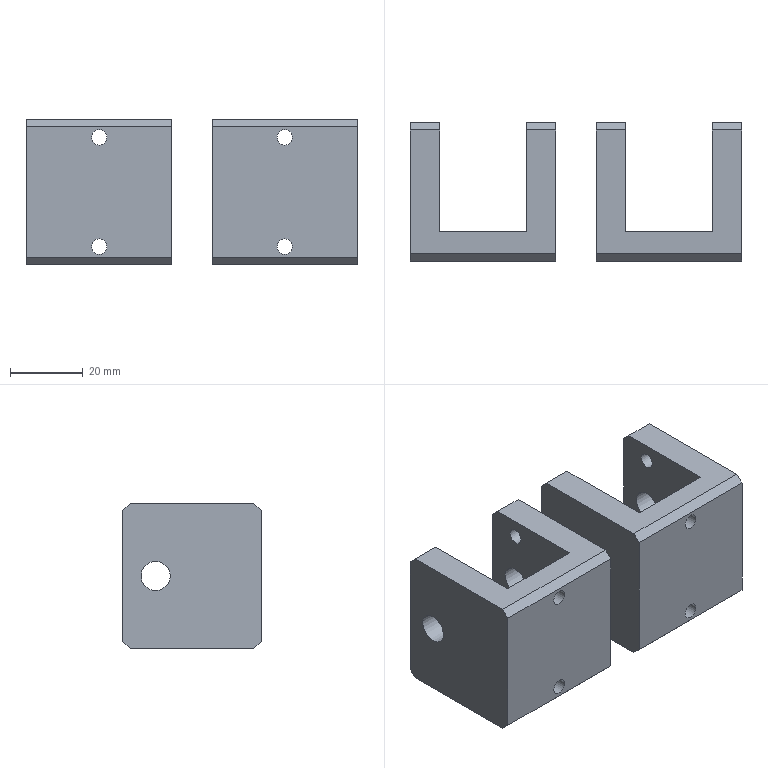NC program | NX | posted by the shop | part box 91 x 38 x 40 mm
Lines 1 to 3675 of 4199, first 2229 of 3673 lines:
%
O0001
(Machine time: 136.35 MIN)
(===Total Tool:6===)
(T1=D80R0.8 face mill D=80.  R=0.8  D-  H01 Z=-0.   )
(T9=D10     D=10.  R=0.   D-  H09 Z=-38.1 )
(T2=D6 chamfer mill   D=6.   R=0.   D-  H02 Z=-31.5 )
(T14=Drill 4.2  D=4.2  DR_a=118 D-  H14 Z=-45.26)
(T10=D10-J  D=10.  R=0.   D-  H10 Z=-38.  )
(T22=M5X0.8 D=4.2  DR_a=180 D-  H22 Z=-41.5 )
G80 G90 G17 G49 G40
G91 G28 Z0
M01
N1 T01 M06
(D80R0.8 face mill  D=80. R=0.8 H=01 ce=0.00 di=0.00)
G00 G90 G54 X90.5 Y0.0 M03 S4000
G43 H01 Z50.
M08
Z2.
G01 Z0.0 F1000.
X85.5
X-85.5
X-90.5
Z2.
G00 Z50.
G91 G28 Z0.0
M05
M09
G91 G28 Z0.0
M01
N2 T09 M06
(D10  D=10. R=0. H=09 ce=0.10 di=0.00)
G00 G90 G54 X50.6 Y0.0 M03 S8000
G43 H09 Z50.
M08
Z.5
G01 Y-20. Z.418 F5000.
G02 X45.5 Y-25.1 Z.385 I-5.1 J0.0
G01 X5.5 Z.221
G02 X.4 Y-20. Z.188 I0.0 J5.1
G01 Y20. Z.024
G02 X5.5 Y25.1 Z-.009 I5.1 J0.0
G01 X45.5 Z-.173
G02 X50.6 Y20. Z-.206 I0.0 J-5.1
G01 Y-20. Z-.37
G02 X45.5 Y-25.1 Z-.403 I-5.1 J0.0
G01 X5.5 Z-.567
G02 X.4 Y-20. Z-.6 I0.0 J5.1
G01 Y20. Z-.764
G02 X5.5 Y25.1 Z-.797 I5.1 J0.0
G01 X45.5 Z-.961
G02 X50.6 Y20. Z-.993 I0.0 J-5.1
G01 Y-20. Z-1.158
G02 X45.5 Y-25.1 Z-1.19 I-5.1 J0.0
G01 X5.5 Z-1.354
G02 X.4 Y-20. Z-1.387 I0.0 J5.1
G01 Y20. Z-1.551
G02 X5.5 Y25.1 Z-1.584 I5.1 J0.0
G01 X45.5 Z-1.748
G02 X50.6 Y20. Z-1.781 I0.0 J-5.1
G01 Y-20. Z-1.945
G02 X45.5 Y-25.1 Z-1.978 I-5.1 J0.0
G01 X5.5 Z-2.142
G02 X.4 Y-20. Z-2.175 I0.0 J5.1
G01 Y20. Z-2.339
G02 X5.5 Y25.1 Z-2.372 I5.1 J0.0
G01 X45.5 Z-2.536
G02 X50.6 Y20. Z-2.569 I0.0 J-5.1
G01 Y-20. Z-2.733
G02 X45.5 Y-25.1 Z-2.766 I-5.1 J0.0
G01 X5.5 Z-2.93
G02 X.4 Y-20. Z-2.963 I0.0 J5.1
G01 Y20. Z-3.127
G02 X5.5 Y25.1 Z-3.16 I5.1 J0.0
G01 X45.5 Z-3.324
G02 X50.6 Y20. Z-3.357 I0.0 J-5.1
G01 Y-20. Z-3.521
G02 X45.5 Y-25.1 Z-3.554 I-5.1 J0.0
G01 X5.5 Z-3.718
G02 X.4 Y-20. Z-3.751 I0.0 J5.1
G01 Y20. Z-3.915
G02 X5.5 Y25.1 Z-3.948 I5.1 J0.0
G01 X45.5 Z-4.112
G02 X50.6 Y20. Z-4.144 I0.0 J-5.1
G01 Y-20. Z-4.309
G02 X45.5 Y-25.1 Z-4.341 I-5.1 J0.0
G01 X5.5 Z-4.506
G02 X.4 Y-20. Z-4.538 I0.0 J5.1
G01 Y20. Z-4.702
G02 X5.5 Y25.1 Z-4.735 I5.1 J0.0
G01 X45.5 Z-4.899
G02 X50.6 Y20. Z-4.932 I0.0 J-5.1
G01 Y-20. Z-5.096
G02 X45.5 Y-25.1 Z-5.129 I-5.1 J0.0
G01 X5.5 Z-5.293
G02 X.4 Y-20. Z-5.326 I0.0 J5.1
G01 Y20. Z-5.49
G02 X5.5 Y25.1 Z-5.523 I5.1 J0.0
G01 X45.5 Z-5.687
G02 X50.6 Y20. Z-5.72 I0.0 J-5.1
G01 Y-20. Z-5.884
G02 X45.5 Y-25.1 Z-5.917 I-5.1 J0.0
G01 X5.5 Z-6.081
G02 X.4 Y-20. Z-6.114 I0.0 J5.1
G01 Y20. Z-6.278
G02 X5.5 Y25.1 Z-6.311 I5.1 J0.0
G01 X45.5 Z-6.475
G02 X50.6 Y20. Z-6.508 I0.0 J-5.1
G01 Y-20. Z-6.672
G02 X45.5 Y-25.1 Z-6.705 I-5.1 J0.0
G01 X5.5 Z-6.869
G02 X.4 Y-20. Z-6.902 I0.0 J5.1
G01 Y20. Z-7.066
G02 X5.5 Y25.1 Z-7.099 I5.1 J0.0
G01 X45.5 Z-7.263
G02 X50.6 Y20. Z-7.296 I0.0 J-5.1
G01 Y-20. Z-7.46
G02 X45.5 Y-25.1 Z-7.492 I-5.1 J0.0
G01 X5.5 Z-7.657
G02 X.4 Y-20. Z-7.689 I0.0 J5.1
G01 Y20. Z-7.853
G02 X5.5 Y25.1 Z-7.886 I5.1 J0.0
G01 X45.5 Z-8.05
G02 X50.6 Y20. Z-8.083 I0.0 J-5.1
G01 Y-20. Z-8.247
G02 X45.5 Y-25.1 Z-8.28 I-5.1 J0.0
G01 X5.5 Z-8.444
G02 X.4 Y-20. Z-8.477 I0.0 J5.1
G01 Y20. Z-8.641
G02 X5.5 Y25.1 Z-8.674 I5.1 J0.0
G01 X45.5 Z-8.838
G02 X50.6 Y20. Z-8.871 I0.0 J-5.1
G01 Y-20. Z-9.035
G02 X45.5 Y-25.1 Z-9.068 I-5.1 J0.0
G01 X5.5 Z-9.232
G02 X.4 Y-20. Z-9.265 I0.0 J5.1
G01 Y20. Z-9.429
G02 X5.5 Y25.1 Z-9.462 I5.1 J0.0
G01 X45.5 Z-9.626
G02 X50.6 Y20. Z-9.659 I0.0 J-5.1
G01 Y-20. Z-9.823
G02 X45.5 Y-25.1 Z-9.856 I-5.1 J0.0
G01 X5.5 Z-10.02
G02 X.4 Y-20. Z-10.053 I0.0 J5.1
G01 Y20. Z-10.217
G02 X5.5 Y25.1 Z-10.25 I5.1 J0.0
G01 X45.5 Z-10.414
G02 X50.6 Y20. Z-10.447 I0.0 J-5.1
G01 Y-20. Z-10.611
G02 X45.5 Y-25.1 Z-10.643 I-5.1 J0.0
G01 X5.5 Z-10.808
G02 X.4 Y-20. Z-10.84 I0.0 J5.1
G01 Y20. Z-11.004
G02 X5.5 Y25.1 Z-11.037 I5.1 J0.0
G01 X45.5 Z-11.201
G02 X50.6 Y20. Z-11.234 I0.0 J-5.1
G01 Y-20. Z-11.398
G02 X45.5 Y-25.1 Z-11.431 I-5.1 J0.0
G01 X5.5 Z-11.595
G02 X.4 Y-20. Z-11.628 I0.0 J5.1
G01 Y20. Z-11.792
G02 X5.5 Y25.1 Z-11.825 I5.1 J0.0
G01 X45.5 Z-11.989
G02 X50.6 Y20. Z-12.022 I0.0 J-5.1
G01 Y-20. Z-12.186
G02 X45.5 Y-25.1 Z-12.219 I-5.1 J0.0
G01 X5.5 Z-12.383
G02 X.4 Y-20. Z-12.416 I0.0 J5.1
G01 Y20. Z-12.58
G02 X5.5 Y25.1 Z-12.613 I5.1 J0.0
G01 X45.5 Z-12.777
G02 X50.6 Y20. Z-12.81 I0.0 J-5.1
G01 Y-20. Z-12.974
G02 X45.5 Y-25.1 Z-13.007 I-5.1 J0.0
G01 X5.5 Z-13.171
G02 X.4 Y-20. Z-13.204 I0.0 J5.1
G01 Y20. Z-13.368
G02 X5.5 Y25.1 Z-13.401 I5.1 J0.0
G01 X45.5 Z-13.565
G02 X50.6 Y20. Z-13.598 I0.0 J-5.1
G01 Y-20. Z-13.762
G02 X45.5 Y-25.1 Z-13.794 I-5.1 J0.0
G01 X5.5 Z-13.959
G02 X.4 Y-20. Z-13.991 I0.0 J5.1
G01 Y20. Z-14.156
G02 X5.5 Y25.1 Z-14.188 I5.1 J0.0
G01 X45.5 Z-14.352
G02 X50.6 Y20. Z-14.385 I0.0 J-5.1
G01 Y-20. Z-14.549
G02 X45.5 Y-25.1 Z-14.582 I-5.1 J0.0
G01 X5.5 Z-14.746
G02 X.4 Y-20. Z-14.779 I0.0 J5.1
G01 Y20. Z-14.943
G02 X5.5 Y25.1 Z-14.976 I5.1 J0.0
G01 X45.5 Z-15.14
G02 X50.6 Y20. Z-15.173 I0.0 J-5.1
G01 Y-20. Z-15.337
G02 X45.5 Y-25.1 Z-15.37 I-5.1 J0.0
G01 X5.5 Z-15.534
G02 X.4 Y-20. Z-15.567 I0.0 J5.1
G01 Y20. Z-15.731
G02 X5.5 Y25.1 Z-15.764 I5.1 J0.0
G01 X45.5 Z-15.928
G02 X50.6 Y20. Z-15.961 I0.0 J-5.1
G01 Y-20. Z-16.125
G02 X45.5 Y-25.1 Z-16.158 I-5.1 J0.0
G01 X5.5 Z-16.322
G02 X.4 Y-20. Z-16.355 I0.0 J5.1
G01 Y20. Z-16.519
G02 X5.5 Y25.1 Z-16.552 I5.1 J0.0
G01 X45.5 Z-16.716
G02 X50.6 Y20. Z-16.749 I0.0 J-5.1
G01 Y-20. Z-16.913
G02 X45.5 Y-25.1 Z-16.946 I-5.1 J0.0
G01 X5.5 Z-17.11
G02 X.4 Y-20. Z-17.142 I0.0 J5.1
G01 Y20. Z-17.307
G02 X5.5 Y25.1 Z-17.339 I5.1 J0.0
G01 X45.5 Z-17.503
G02 X50.6 Y20. Z-17.536 I0.0 J-5.1
G01 Y-20. Z-17.7
G02 X45.5 Y-25.1 Z-17.733 I-5.1 J0.0
G01 X5.5 Z-17.897
G02 X.4 Y-20. Z-17.93 I0.0 J5.1
G01 Y20. Z-18.094
G02 X5.5 Y25.1 Z-18.127 I5.1 J0.0
G01 X45.5 Z-18.291
G02 X50.6 Y20. Z-18.324 I0.0 J-5.1
G01 Y-20. Z-18.488
G02 X45.5 Y-25.1 Z-18.521 I-5.1 J0.0
G01 X5.5 Z-18.685
G02 X.4 Y-20. Z-18.718 I0.0 J5.1
G01 Y20. Z-18.882
G02 X5.5 Y25.1 Z-18.915 I5.1 J0.0
G01 X45.5 Z-19.079
G02 X50.6 Y20. Z-19.112 I0.0 J-5.1
G01 Y-20. Z-19.276
G02 X45.5 Y-25.1 Z-19.309 I-5.1 J0.0
G01 X5.5 Z-19.473
G02 X.4 Y-20. Z-19.506 I0.0 J5.1
G01 Y20. Z-19.67
G02 X5.5 Y25.1 Z-19.703 I5.1 J0.0
G01 X45.5 Z-19.867
G02 X50.6 Y20. Z-19.9 I0.0 J-5.1
G01 Y-20. Z-20.064
G02 X45.5 Y-25.1 Z-20.097 I-5.1 J0.0
G01 X5.5 Z-20.261
G02 X.4 Y-20. Z-20.293 I0.0 J5.1
G01 Y20. Z-20.458
G02 X5.5 Y25.1 Z-20.49 I5.1 J0.0
G01 X45.5 Z-20.654
G02 X50.6 Y20. Z-20.687 I0.0 J-5.1
G01 Y-20. Z-20.851
G02 X45.5 Y-25.1 Z-20.884 I-5.1 J0.0
G01 X5.5 Z-21.048
G02 X.4 Y-20. Z-21.081 I0.0 J5.1
G01 Y20. Z-21.245
G02 X5.5 Y25.1 Z-21.278 I5.1 J0.0
G01 X45.5 Z-21.442
G02 X50.6 Y20. Z-21.475 I0.0 J-5.1
G01 Y-20. Z-21.639
G02 X45.5 Y-25.1 Z-21.672 I-5.1 J0.0
G01 X5.5 Z-21.836
G02 X.4 Y-20. Z-21.869 I0.0 J5.1
G01 Y20. Z-22.033
G02 X5.5 Y25.1 Z-22.066 I5.1 J0.0
G01 X45.5 Z-22.23
G02 X50.6 Y20. Z-22.263 I0.0 J-5.1
G01 Y-20. Z-22.427
G02 X45.5 Y-25.1 Z-22.46 I-5.1 J0.0
G01 X5.5 Z-22.624
G02 X.4 Y-20. Z-22.657 I0.0 J5.1
G01 Y20. Z-22.821
G02 X5.5 Y25.1 Z-22.854 I5.1 J0.0
G01 X45.5 Z-23.018
G02 X50.6 Y20. Z-23.051 I0.0 J-5.1
G01 Y-20. Z-23.215
G02 X45.5 Y-25.1 Z-23.248 I-5.1 J0.0
G01 X5.5 Z-23.412
G02 X.4 Y-20. Z-23.444 I0.0 J5.1
G01 Y20. Z-23.609
G02 X5.5 Y25.1 Z-23.641 I5.1 J0.0
G01 X45.5 Z-23.806
G02 X50.6 Y20. Z-23.838 I0.0 J-5.1
G01 Y-20. Z-24.002
G02 X45.5 Y-25.1 Z-24.035 I-5.1 J0.0
G01 X5.5 Z-24.199
G02 X.4 Y-20. Z-24.232 I0.0 J5.1
G01 Y20. Z-24.396
G02 X5.5 Y25.1 Z-24.429 I5.1 J0.0
G01 X45.5 Z-24.593
G02 X50.6 Y20. Z-24.626 I0.0 J-5.1
G01 Y-20. Z-24.79
G02 X45.5 Y-25.1 Z-24.823 I-5.1 J0.0
G01 X5.5 Z-24.987
G02 X.4 Y-20. Z-25.02 I0.0 J5.1
G01 Y20. Z-25.184
G02 X5.5 Y25.1 Z-25.217 I5.1 J0.0
G01 X45.5 Z-25.381
G02 X50.6 Y20. Z-25.414 I0.0 J-5.1
G01 Y-20. Z-25.578
G02 X45.5 Y-25.1 Z-25.611 I-5.1 J0.0
G01 X5.5 Z-25.775
G02 X.4 Y-20. Z-25.808 I0.0 J5.1
G01 Y20. Z-25.972
G02 X5.5 Y25.1 Z-26.005 I5.1 J0.0
G01 X45.5 Z-26.169
G02 X50.6 Y20. Z-26.202 I0.0 J-5.1
G01 Y-20. Z-26.366
G02 X45.5 Y-25.1 Z-26.399 I-5.1 J0.0
G01 X5.5 Z-26.563
G02 X.4 Y-20. Z-26.596 I0.0 J5.1
G01 Y20. Z-26.76
G02 X5.5 Y25.1 Z-26.792 I5.1 J0.0
G01 X45.5 Z-26.957
G02 X50.6 Y20. Z-26.989 I0.0 J-5.1
G01 Y-20. Z-27.153
G02 X45.5 Y-25.1 Z-27.186 I-5.1 J0.0
G01 X5.5 Z-27.35
G02 X.4 Y-20. Z-27.383 I0.0 J5.1
G01 Y20. Z-27.547
G02 X5.5 Y25.1 Z-27.58 I5.1 J0.0
G01 X45.5 Z-27.744
G02 X50.6 Y20. Z-27.777 I0.0 J-5.1
G01 Y-20. Z-27.941
G02 X45.5 Y-25.1 Z-27.974 I-5.1 J0.0
G01 X5.5 Z-28.138
G02 X.4 Y-20. Z-28.171 I0.0 J5.1
G01 Y20. Z-28.335
G02 X5.5 Y25.1 Z-28.368 I5.1 J0.0
G01 X45.5 Z-28.532
G02 X50.6 Y20. Z-28.565 I0.0 J-5.1
G01 Y-20. Z-28.729
G02 X45.5 Y-25.1 Z-28.762 I-5.1 J0.0
G01 X5.5 Z-28.926
G02 X.4 Y-20. Z-28.959 I0.0 J5.1
G01 Y20. Z-29.123
G02 X5.5 Y25.1 Z-29.156 I5.1 J0.0
G01 X45.5 Z-29.32
G02 X50.6 Y20. Z-29.353 I0.0 J-5.1
G01 Y-20. Z-29.517
G02 X45.5 Y-25.1 Z-29.55 I-5.1 J0.0
G01 X5.5 Z-29.714
G02 X.4 Y-20. Z-29.747 I0.0 J5.1
G01 Y20. Z-29.911
G02 X5.5 Y25.1 Z-29.943 I5.1 J0.0
G01 X45.5 Z-30.108
G02 X50.6 Y20. Z-30.14 I0.0 J-5.1
G01 Y-20. Z-30.304
G02 X45.5 Y-25.1 Z-30.337 I-5.1 J0.0
G01 X5.5 Z-30.501
G02 X.4 Y-20. Z-30.534 I0.0 J5.1
G01 Y20. Z-30.698
G02 X5.5 Y25.1 Z-30.731 I5.1 J0.0
G01 X45.5 Z-30.895
G02 X50.6 Y20. Z-30.928 I0.0 J-5.1
G01 Y-20. Z-31.092
G02 X45.5 Y-25.1 Z-31.125 I-5.1 J0.0
G01 X5.5 Z-31.289
G02 X.4 Y-20. Z-31.322 I0.0 J5.1
G01 Y20. Z-31.486
G02 X5.5 Y25.1 Z-31.519 I5.1 J0.0
G01 X45.5 Z-31.683
G02 X50.6 Y20. Z-31.716 I0.0 J-5.1
G01 Y-20. Z-31.88
G02 X45.5 Y-25.1 Z-31.913 I-5.1 J0.0
G01 X5.5 Z-32.077
G02 X.4 Y-20. Z-32.11 I0.0 J5.1
G01 Y20. Z-32.274
G02 X5.5 Y25.1 Z-32.307 I5.1 J0.0
G01 X45.5 Z-32.471
G02 X50.6 Y20. Z-32.504 I0.0 J-5.1
G01 Y-20. Z-32.668
G02 X45.5 Y-25.1 Z-32.701 I-5.1 J0.0
G01 X5.5 Z-32.865
G02 X.4 Y-20. Z-32.898 I0.0 J5.1
G01 Y20. Z-33.062
G02 X5.5 Y25.1 Z-33.094 I5.1 J0.0
G01 X45.5 Z-33.259
G02 X50.6 Y20. Z-33.291 I0.0 J-5.1
G01 Y-20. Z-33.456
G02 X45.5 Y-25.1 Z-33.488 I-5.1 J0.0
G01 X5.5 Z-33.652
G02 X.4 Y-20. Z-33.685 I0.0 J5.1
G01 Y20. Z-33.849
G02 X5.5 Y25.1 Z-33.882 I5.1 J0.0
G01 X45.5 Z-34.046
G02 X50.6 Y20. Z-34.079 I0.0 J-5.1
G01 Y-20. Z-34.243
G02 X45.5 Y-25.1 Z-34.276 I-5.1 J0.0
G01 X5.5 Z-34.44
G02 X.4 Y-20. Z-34.473 I0.0 J5.1
G01 Y20. Z-34.637
G02 X5.5 Y25.1 Z-34.67 I5.1 J0.0
G01 X45.5 Z-34.834
G02 X50.6 Y20. Z-34.867 I0.0 J-5.1
G01 Y-20. Z-35.031
G02 X45.5 Y-25.1 Z-35.064 I-5.1 J0.0
G01 X5.5 Z-35.228
G02 X.4 Y-20. Z-35.261 I0.0 J5.1
G01 Y20. Z-35.425
G02 X5.5 Y25.1 Z-35.458 I5.1 J0.0
G01 X45.5 Z-35.622
G02 X50.6 Y20. Z-35.655 I0.0 J-5.1
G01 Y-20. Z-35.819
G02 X45.5 Y-25.1 Z-35.852 I-5.1 J0.0
G01 X5.5 Z-36.016
G02 X.4 Y-20. Z-36.049 I0.0 J5.1
G01 Y20. Z-36.213
G02 X5.5 Y25.1 Z-36.246 I5.1 J0.0
G01 X45.5 Z-36.41
G02 X50.6 Y20. Z-36.442 I0.0 J-5.1
G01 Y-20. Z-36.607
G02 X45.5 Y-25.1 Z-36.639 I-5.1 J0.0
G01 X5.5 Z-36.803
G02 X.4 Y-20. Z-36.836 I0.0 J5.1
G01 Y20. Z-37.
G02 X5.5 Y25.1 Z-37.033 I5.1 J0.0
G01 X45.5 Z-37.197
G02 X50.6 Y20. Z-37.23 I0.0 J-5.1
G01 Y-20. Z-37.394
G02 X45.5 Y-25.1 Z-37.427 I-5.1 J0.0
G01 X5.5 Z-37.591
G02 X.4 Y-20. Z-37.624 I0.0 J5.1
G01 Y20. Z-37.788
G02 X5.5 Y25.1 Z-37.821 I5.1 J0.0
G01 X45.5 Z-37.985
G02 X50.6 Y20. Z-38.018 I0.0 J-5.1
G01 Y0.0 Z-38.1
Y-20.
G02 X45.5 Y-25.1 I-5.1 J0.0
G01 X5.5
G02 X.4 Y-20. I0.0 J5.1
G01 Y20.
G02 X5.5 Y25.1 I5.1 J0.0
G01 X45.5
G02 X50.6 Y20. I0.0 J-5.1
G01 Y0.0
Y-.5
Z-37.1
G00 Z50.
X-25.5 Y25.1
Z.5
G01 X-5.5 Z.418
G02 X-.4 Y20. Z.385 I0.0 J-5.1
G01 Y-20. Z.221
G02 X-5.5 Y-25.1 Z.188 I-5.1 J0.0
G01 X-45.5 Z.024
G02 X-50.6 Y-20. Z-.009 I0.0 J5.1
G01 Y20. Z-.173
G02 X-45.5 Y25.1 Z-.206 I5.1 J0.0
G01 X-5.5 Z-.37
G02 X-.4 Y20. Z-.403 I0.0 J-5.1
G01 Y-20. Z-.567
G02 X-5.5 Y-25.1 Z-.6 I-5.1 J0.0
G01 X-45.5 Z-.764
G02 X-50.6 Y-20. Z-.797 I0.0 J5.1
G01 Y20. Z-.961
G02 X-45.5 Y25.1 Z-.993 I5.1 J0.0
G01 X-5.5 Z-1.158
G02 X-.4 Y20. Z-1.19 I0.0 J-5.1
G01 Y-20. Z-1.354
G02 X-5.5 Y-25.1 Z-1.387 I-5.1 J0.0
G01 X-45.5 Z-1.551
G02 X-50.6 Y-20. Z-1.584 I0.0 J5.1
G01 Y20. Z-1.748
G02 X-45.5 Y25.1 Z-1.781 I5.1 J0.0
G01 X-5.5 Z-1.945
G02 X-.4 Y20. Z-1.978 I0.0 J-5.1
G01 Y-20. Z-2.142
G02 X-5.5 Y-25.1 Z-2.175 I-5.1 J0.0
G01 X-45.5 Z-2.339
G02 X-50.6 Y-20. Z-2.372 I0.0 J5.1
G01 Y20. Z-2.536
G02 X-45.5 Y25.1 Z-2.569 I5.1 J0.0
G01 X-5.5 Z-2.733
G02 X-.4 Y20. Z-2.766 I0.0 J-5.1
G01 Y-20. Z-2.93
G02 X-5.5 Y-25.1 Z-2.963 I-5.1 J0.0
G01 X-45.5 Z-3.127
G02 X-50.6 Y-20. Z-3.16 I0.0 J5.1
G01 Y20. Z-3.324
G02 X-45.5 Y25.1 Z-3.357 I5.1 J0.0
G01 X-5.5 Z-3.521
G02 X-.4 Y20. Z-3.554 I0.0 J-5.1
G01 Y-20. Z-3.718
G02 X-5.5 Y-25.1 Z-3.751 I-5.1 J0.0
G01 X-45.5 Z-3.915
G02 X-50.6 Y-20. Z-3.948 I0.0 J5.1
G01 Y20. Z-4.112
G02 X-45.5 Y25.1 Z-4.144 I5.1 J0.0
G01 X-5.5 Z-4.309
G02 X-.4 Y20. Z-4.341 I0.0 J-5.1
G01 Y-20. Z-4.506
G02 X-5.5 Y-25.1 Z-4.538 I-5.1 J0.0
G01 X-45.5 Z-4.702
G02 X-50.6 Y-20. Z-4.735 I0.0 J5.1
G01 Y20. Z-4.899
G02 X-45.5 Y25.1 Z-4.932 I5.1 J0.0
G01 X-5.5 Z-5.096
G02 X-.4 Y20. Z-5.129 I0.0 J-5.1
G01 Y-20. Z-5.293
G02 X-5.5 Y-25.1 Z-5.326 I-5.1 J0.0
G01 X-45.5 Z-5.49
G02 X-50.6 Y-20. Z-5.523 I0.0 J5.1
G01 Y20. Z-5.687
G02 X-45.5 Y25.1 Z-5.72 I5.1 J0.0
G01 X-5.5 Z-5.884
G02 X-.4 Y20. Z-5.917 I0.0 J-5.1
G01 Y-20. Z-6.081
G02 X-5.5 Y-25.1 Z-6.114 I-5.1 J0.0
G01 X-45.5 Z-6.278
G02 X-50.6 Y-20. Z-6.311 I0.0 J5.1
G01 Y20. Z-6.475
G02 X-45.5 Y25.1 Z-6.508 I5.1 J0.0
G01 X-5.5 Z-6.672
G02 X-.4 Y20. Z-6.705 I0.0 J-5.1
G01 Y-20. Z-6.869
G02 X-5.5 Y-25.1 Z-6.902 I-5.1 J0.0
G01 X-45.5 Z-7.066
G02 X-50.6 Y-20. Z-7.099 I0.0 J5.1
G01 Y20. Z-7.263
G02 X-45.5 Y25.1 Z-7.296 I5.1 J0.0
G01 X-5.5 Z-7.46
G02 X-.4 Y20. Z-7.492 I0.0 J-5.1
G01 Y-20. Z-7.657
G02 X-5.5 Y-25.1 Z-7.689 I-5.1 J0.0
G01 X-45.5 Z-7.853
G02 X-50.6 Y-20. Z-7.886 I0.0 J5.1
G01 Y20. Z-8.05
G02 X-45.5 Y25.1 Z-8.083 I5.1 J0.0
G01 X-5.5 Z-8.247
G02 X-.4 Y20. Z-8.28 I0.0 J-5.1
G01 Y-20. Z-8.444
G02 X-5.5 Y-25.1 Z-8.477 I-5.1 J0.0
G01 X-45.5 Z-8.641
G02 X-50.6 Y-20. Z-8.674 I0.0 J5.1
G01 Y20. Z-8.838
G02 X-45.5 Y25.1 Z-8.871 I5.1 J0.0
G01 X-5.5 Z-9.035
G02 X-.4 Y20. Z-9.068 I0.0 J-5.1
G01 Y-20. Z-9.232
G02 X-5.5 Y-25.1 Z-9.265 I-5.1 J0.0
G01 X-45.5 Z-9.429
G02 X-50.6 Y-20. Z-9.462 I0.0 J5.1
G01 Y20. Z-9.626
G02 X-45.5 Y25.1 Z-9.659 I5.1 J0.0
G01 X-5.5 Z-9.823
G02 X-.4 Y20. Z-9.856 I0.0 J-5.1
G01 Y-20. Z-10.02
G02 X-5.5 Y-25.1 Z-10.053 I-5.1 J0.0
G01 X-45.5 Z-10.217
G02 X-50.6 Y-20. Z-10.25 I0.0 J5.1
G01 Y20. Z-10.414
G02 X-45.5 Y25.1 Z-10.447 I5.1 J0.0
G01 X-5.5 Z-10.611
G02 X-.4 Y20. Z-10.643 I0.0 J-5.1
G01 Y-20. Z-10.808
G02 X-5.5 Y-25.1 Z-10.84 I-5.1 J0.0
G01 X-45.5 Z-11.004
G02 X-50.6 Y-20. Z-11.037 I0.0 J5.1
G01 Y20. Z-11.201
G02 X-45.5 Y25.1 Z-11.234 I5.1 J0.0
G01 X-5.5 Z-11.398
G02 X-.4 Y20. Z-11.431 I0.0 J-5.1
G01 Y-20. Z-11.595
G02 X-5.5 Y-25.1 Z-11.628 I-5.1 J0.0
G01 X-45.5 Z-11.792
G02 X-50.6 Y-20. Z-11.825 I0.0 J5.1
G01 Y20. Z-11.989
G02 X-45.5 Y25.1 Z-12.022 I5.1 J0.0
G01 X-5.5 Z-12.186
G02 X-.4 Y20. Z-12.219 I0.0 J-5.1
G01 Y-20. Z-12.383
G02 X-5.5 Y-25.1 Z-12.416 I-5.1 J0.0
G01 X-45.5 Z-12.58
G02 X-50.6 Y-20. Z-12.613 I0.0 J5.1
G01 Y20. Z-12.777
G02 X-45.5 Y25.1 Z-12.81 I5.1 J0.0
G01 X-5.5 Z-12.974
G02 X-.4 Y20. Z-13.007 I0.0 J-5.1
G01 Y-20. Z-13.171
G02 X-5.5 Y-25.1 Z-13.204 I-5.1 J0.0
G01 X-45.5 Z-13.368
G02 X-50.6 Y-20. Z-13.401 I0.0 J5.1
G01 Y20. Z-13.565
G02 X-45.5 Y25.1 Z-13.598 I5.1 J0.0
G01 X-5.5 Z-13.762
G02 X-.4 Y20. Z-13.794 I0.0 J-5.1
G01 Y-20. Z-13.959
G02 X-5.5 Y-25.1 Z-13.991 I-5.1 J0.0
G01 X-45.5 Z-14.156
G02 X-50.6 Y-20. Z-14.188 I0.0 J5.1
G01 Y20. Z-14.352
G02 X-45.5 Y25.1 Z-14.385 I5.1 J0.0
G01 X-5.5 Z-14.549
G02 X-.4 Y20. Z-14.582 I0.0 J-5.1
G01 Y-20. Z-14.746
G02 X-5.5 Y-25.1 Z-14.779 I-5.1 J0.0
G01 X-45.5 Z-14.943
G02 X-50.6 Y-20. Z-14.976 I0.0 J5.1
G01 Y20. Z-15.14
G02 X-45.5 Y25.1 Z-15.173 I5.1 J0.0
G01 X-5.5 Z-15.337
G02 X-.4 Y20. Z-15.37 I0.0 J-5.1
G01 Y-20. Z-15.534
G02 X-5.5 Y-25.1 Z-15.567 I-5.1 J0.0
G01 X-45.5 Z-15.731
G02 X-50.6 Y-20. Z-15.764 I0.0 J5.1
G01 Y20. Z-15.928
G02 X-45.5 Y25.1 Z-15.961 I5.1 J0.0
G01 X-5.5 Z-16.125
G02 X-.4 Y20. Z-16.158 I0.0 J-5.1
G01 Y-20. Z-16.322
G02 X-5.5 Y-25.1 Z-16.355 I-5.1 J0.0
G01 X-45.5 Z-16.519
G02 X-50.6 Y-20. Z-16.552 I0.0 J5.1
G01 Y20. Z-16.716
G02 X-45.5 Y25.1 Z-16.749 I5.1 J0.0
G01 X-5.5 Z-16.913
G02 X-.4 Y20. Z-16.946 I0.0 J-5.1
G01 Y-20. Z-17.11
G02 X-5.5 Y-25.1 Z-17.142 I-5.1 J0.0
G01 X-45.5 Z-17.307
G02 X-50.6 Y-20. Z-17.339 I0.0 J5.1
G01 Y20. Z-17.503
G02 X-45.5 Y25.1 Z-17.536 I5.1 J0.0
G01 X-5.5 Z-17.7
G02 X-.4 Y20. Z-17.733 I0.0 J-5.1
G01 Y-20. Z-17.897
G02 X-5.5 Y-25.1 Z-17.93 I-5.1 J0.0
G01 X-45.5 Z-18.094
G02 X-50.6 Y-20. Z-18.127 I0.0 J5.1
G01 Y20. Z-18.291
G02 X-45.5 Y25.1 Z-18.324 I5.1 J0.0
G01 X-5.5 Z-18.488
G02 X-.4 Y20. Z-18.521 I0.0 J-5.1
G01 Y-20. Z-18.685
G02 X-5.5 Y-25.1 Z-18.718 I-5.1 J0.0
G01 X-45.5 Z-18.882
G02 X-50.6 Y-20. Z-18.915 I0.0 J5.1
G01 Y20. Z-19.079
G02 X-45.5 Y25.1 Z-19.112 I5.1 J0.0
G01 X-5.5 Z-19.276
G02 X-.4 Y20. Z-19.309 I0.0 J-5.1
G01 Y-20. Z-19.473
G02 X-5.5 Y-25.1 Z-19.506 I-5.1 J0.0
G01 X-45.5 Z-19.67
G02 X-50.6 Y-20. Z-19.703 I0.0 J5.1
G01 Y20. Z-19.867
G02 X-45.5 Y25.1 Z-19.9 I5.1 J0.0
G01 X-5.5 Z-20.064
G02 X-.4 Y20. Z-20.097 I0.0 J-5.1
G01 Y-20. Z-20.261
G02 X-5.5 Y-25.1 Z-20.293 I-5.1 J0.0
G01 X-45.5 Z-20.458
G02 X-50.6 Y-20. Z-20.49 I0.0 J5.1
G01 Y20. Z-20.654
G02 X-45.5 Y25.1 Z-20.687 I5.1 J0.0
G01 X-5.5 Z-20.851
G02 X-.4 Y20. Z-20.884 I0.0 J-5.1
G01 Y-20. Z-21.048
G02 X-5.5 Y-25.1 Z-21.081 I-5.1 J0.0
G01 X-45.5 Z-21.245
G02 X-50.6 Y-20. Z-21.278 I0.0 J5.1
G01 Y20. Z-21.442
G02 X-45.5 Y25.1 Z-21.475 I5.1 J0.0
G01 X-5.5 Z-21.639
G02 X-.4 Y20. Z-21.672 I0.0 J-5.1
G01 Y-20. Z-21.836
G02 X-5.5 Y-25.1 Z-21.869 I-5.1 J0.0
G01 X-45.5 Z-22.033
G02 X-50.6 Y-20. Z-22.066 I0.0 J5.1
G01 Y20. Z-22.23
G02 X-45.5 Y25.1 Z-22.263 I5.1 J0.0
G01 X-5.5 Z-22.427
G02 X-.4 Y20. Z-22.46 I0.0 J-5.1
G01 Y-20. Z-22.624
G02 X-5.5 Y-25.1 Z-22.657 I-5.1 J0.0
G01 X-45.5 Z-22.821
G02 X-50.6 Y-20. Z-22.854 I0.0 J5.1
G01 Y20. Z-23.018
G02 X-45.5 Y25.1 Z-23.051 I5.1 J0.0
G01 X-5.5 Z-23.215
G02 X-.4 Y20. Z-23.248 I0.0 J-5.1
G01 Y-20. Z-23.412
G02 X-5.5 Y-25.1 Z-23.444 I-5.1 J0.0
G01 X-45.5 Z-23.609
G02 X-50.6 Y-20. Z-23.641 I0.0 J5.1
G01 Y20. Z-23.806
G02 X-45.5 Y25.1 Z-23.838 I5.1 J0.0
G01 X-5.5 Z-24.002
G02 X-.4 Y20. Z-24.035 I0.0 J-5.1
G01 Y-20. Z-24.199
G02 X-5.5 Y-25.1 Z-24.232 I-5.1 J0.0
G01 X-45.5 Z-24.396
G02 X-50.6 Y-20. Z-24.429 I0.0 J5.1
G01 Y20. Z-24.593
G02 X-45.5 Y25.1 Z-24.626 I5.1 J0.0
G01 X-5.5 Z-24.79
G02 X-.4 Y20. Z-24.823 I0.0 J-5.1
G01 Y-20. Z-24.987
G02 X-5.5 Y-25.1 Z-25.02 I-5.1 J0.0
G01 X-45.5 Z-25.184
G02 X-50.6 Y-20. Z-25.217 I0.0 J5.1
G01 Y20. Z-25.381
G02 X-45.5 Y25.1 Z-25.414 I5.1 J0.0
G01 X-5.5 Z-25.578
G02 X-.4 Y20. Z-25.611 I0.0 J-5.1
G01 Y-20. Z-25.775
G02 X-5.5 Y-25.1 Z-25.808 I-5.1 J0.0
G01 X-45.5 Z-25.972
G02 X-50.6 Y-20. Z-26.005 I0.0 J5.1
G01 Y20. Z-26.169
G02 X-45.5 Y25.1 Z-26.202 I5.1 J0.0
G01 X-5.5 Z-26.366
G02 X-.4 Y20. Z-26.399 I0.0 J-5.1
G01 Y-20. Z-26.563
G02 X-5.5 Y-25.1 Z-26.596 I-5.1 J0.0
G01 X-45.5 Z-26.76
G02 X-50.6 Y-20. Z-26.792 I0.0 J5.1
G01 Y20. Z-26.957
G02 X-45.5 Y25.1 Z-26.989 I5.1 J0.0
G01 X-5.5 Z-27.153
G02 X-.4 Y20. Z-27.186 I0.0 J-5.1
G01 Y-20. Z-27.35
G02 X-5.5 Y-25.1 Z-27.383 I-5.1 J0.0
G01 X-45.5 Z-27.547
G02 X-50.6 Y-20. Z-27.58 I0.0 J5.1
G01 Y20. Z-27.744
G02 X-45.5 Y25.1 Z-27.777 I5.1 J0.0
G01 X-5.5 Z-27.941
G02 X-.4 Y20. Z-27.974 I0.0 J-5.1
G01 Y-20. Z-28.138
G02 X-5.5 Y-25.1 Z-28.171 I-5.1 J0.0
G01 X-45.5 Z-28.335
G02 X-50.6 Y-20. Z-28.368 I0.0 J5.1
G01 Y20. Z-28.532
G02 X-45.5 Y25.1 Z-28.565 I5.1 J0.0
G01 X-5.5 Z-28.729
G02 X-.4 Y20. Z-28.762 I0.0 J-5.1
G01 Y-20. Z-28.926
G02 X-5.5 Y-25.1 Z-28.959 I-5.1 J0.0
G01 X-45.5 Z-29.123
G02 X-50.6 Y-20. Z-29.156 I0.0 J5.1
G01 Y20. Z-29.32
G02 X-45.5 Y25.1 Z-29.353 I5.1 J0.0
G01 X-5.5 Z-29.517
G02 X-.4 Y20. Z-29.55 I0.0 J-5.1
G01 Y-20. Z-29.714
G02 X-5.5 Y-25.1 Z-29.747 I-5.1 J0.0
G01 X-45.5 Z-29.911
G02 X-50.6 Y-20. Z-29.943 I0.0 J5.1
G01 Y20. Z-30.108
G02 X-45.5 Y25.1 Z-30.14 I5.1 J0.0
G01 X-5.5 Z-30.304
G02 X-.4 Y20. Z-30.337 I0.0 J-5.1
G01 Y-20. Z-30.501
G02 X-5.5 Y-25.1 Z-30.534 I-5.1 J0.0
G01 X-45.5 Z-30.698
G02 X-50.6 Y-20. Z-30.731 I0.0 J5.1
G01 Y20. Z-30.895
G02 X-45.5 Y25.1 Z-30.928 I5.1 J0.0
G01 X-5.5 Z-31.092
G02 X-.4 Y20. Z-31.125 I0.0 J-5.1
G01 Y-20. Z-31.289
G02 X-5.5 Y-25.1 Z-31.322 I-5.1 J0.0
G01 X-45.5 Z-31.486
G02 X-50.6 Y-20. Z-31.519 I0.0 J5.1
G01 Y20. Z-31.683
G02 X-45.5 Y25.1 Z-31.716 I5.1 J0.0
G01 X-5.5 Z-31.88
G02 X-.4 Y20. Z-31.913 I0.0 J-5.1
G01 Y-20. Z-32.077
G02 X-5.5 Y-25.1 Z-32.11 I-5.1 J0.0
G01 X-45.5 Z-32.274
G02 X-50.6 Y-20. Z-32.307 I0.0 J5.1
G01 Y20. Z-32.471
G02 X-45.5 Y25.1 Z-32.504 I5.1 J0.0
G01 X-5.5 Z-32.668
G02 X-.4 Y20. Z-32.701 I0.0 J-5.1
G01 Y-20. Z-32.865
G02 X-5.5 Y-25.1 Z-32.898 I-5.1 J0.0
G01 X-45.5 Z-33.062
G02 X-50.6 Y-20. Z-33.094 I0.0 J5.1
G01 Y20. Z-33.259
G02 X-45.5 Y25.1 Z-33.291 I5.1 J0.0
G01 X-5.5 Z-33.456
G02 X-.4 Y20. Z-33.488 I0.0 J-5.1
G01 Y-20. Z-33.652
G02 X-5.5 Y-25.1 Z-33.685 I-5.1 J0.0
G01 X-45.5 Z-33.849
G02 X-50.6 Y-20. Z-33.882 I0.0 J5.1
G01 Y20. Z-34.046
G02 X-45.5 Y25.1 Z-34.079 I5.1 J0.0
G01 X-5.5 Z-34.243
G02 X-.4 Y20. Z-34.276 I0.0 J-5.1
G01 Y-20. Z-34.44
G02 X-5.5 Y-25.1 Z-34.473 I-5.1 J0.0
G01 X-45.5 Z-34.637
G02 X-50.6 Y-20. Z-34.67 I0.0 J5.1
G01 Y20. Z-34.834
G02 X-45.5 Y25.1 Z-34.867 I5.1 J0.0
G01 X-5.5 Z-35.031
G02 X-.4 Y20. Z-35.064 I0.0 J-5.1
G01 Y-20. Z-35.228
G02 X-5.5 Y-25.1 Z-35.261 I-5.1 J0.0
G01 X-45.5 Z-35.425
G02 X-50.6 Y-20. Z-35.458 I0.0 J5.1
G01 Y20. Z-35.622
G02 X-45.5 Y25.1 Z-35.655 I5.1 J0.0
G01 X-5.5 Z-35.819
G02 X-.4 Y20. Z-35.852 I0.0 J-5.1
G01 Y-20. Z-36.016
G02 X-5.5 Y-25.1 Z-36.049 I-5.1 J0.0
G01 X-45.5 Z-36.213
G02 X-50.6 Y-20. Z-36.246 I0.0 J5.1
G01 Y20. Z-36.41
G02 X-45.5 Y25.1 Z-36.442 I5.1 J0.0
G01 X-5.5 Z-36.607
G02 X-.4 Y20. Z-36.639 I0.0 J-5.1
G01 Y-20. Z-36.803
G02 X-5.5 Y-25.1 Z-36.836 I-5.1 J0.0
G01 X-45.5 Z-37.
G02 X-50.6 Y-20. Z-37.033 I0.0 J5.1
G01 Y20. Z-37.197
G02 X-45.5 Y25.1 Z-37.23 I5.1 J0.0
G01 X-5.5 Z-37.394
G02 X-.4 Y20. Z-37.427 I0.0 J-5.1
G01 Y-20. Z-37.591
G02 X-5.5 Y-25.1 Z-37.624 I-5.1 J0.0
G01 X-45.5 Z-37.788
G02 X-50.6 Y-20. Z-37.821 I0.0 J5.1
G01 Y20. Z-37.985
G02 X-45.5 Y25.1 Z-38.018 I5.1 J0.0
G01 X-25.5 Z-38.1
X-5.5
G02 X-.4 Y20. I0.0 J-5.1
G01 Y-20.
G02 X-5.5 Y-25.1 I-5.1 J0.0
G01 X-45.5
G02 X-50.6 Y-20. I0.0 J5.1
G01 Y20.
G02 X-45.5 Y25.1 I5.1 J0.0
G01 X-25.5
X-25.
Z-37.1
G00 Z50.
G00 G90 X-25.5 Y-28. M03 S8000
Z50.
Z.002
G01 Z-.498 F3500.
Y-16.5
X-23.1
Y16.5
X-27.9
Y-16.5
X-25.5
Y-21.
X-18.6
Y21.
X-32.4
Y-21.
X-25.5
X-25.
Z.002
G00 Z.5
X-25.5 Y-28.
Z-.497
G01 Z-.997
Y-16.5
X-23.1
Y16.5
X-27.9
Y-16.5
X-25.5
Y-21.
X-18.6
Y21.
X-32.4
Y-21.
X-25.5
X-25.
Z-.497
G00 Z.002
X-25.5 Y-28.
Z-.995
G01 Z-1.495
Y-16.5
X-23.1
Y16.5
X-27.9
Y-16.5
X-25.5
Y-21.
X-18.6
Y21.
X-32.4
Y-21.
X-25.5
X-25.
Z-.995
G00 Z-.497
X-25.5 Y-28.
Z-1.493
G01 Z-1.993
Y-16.5
X-23.1
Y16.5
X-27.9
Y-16.5
X-25.5
Y-21.
X-18.6
Y21.
X-32.4
Y-21.
X-25.5
X-25.
Z-1.493
G00 Z-.995
X-25.5 Y-28.
Z-1.992
G01 Z-2.492
Y-16.5
X-23.1
Y16.5
X-27.9
Y-16.5
X-25.5
Y-21.
X-18.6
Y21.
X-32.4
Y-21.
X-25.5
X-25.
Z-1.992
G00 Z-1.493
X-25.5 Y-28.
Z-2.49
G01 Z-2.99
Y-16.5
X-23.1
Y16.5
X-27.9
Y-16.5
X-25.5
Y-21.
X-18.6
Y21.
X-32.4
Y-21.
X-25.5
X-25.
Z-2.49
G00 Z-1.992
X-25.5 Y-28.
Z-2.988
G01 Z-3.488
Y-16.5
X-23.1
Y16.5
X-27.9
Y-16.5
X-25.5
Y-21.
X-18.6
Y21.
X-32.4
Y-21.
X-25.5
X-25.
Z-2.988
G00 Z-2.49
X-25.5 Y-28.
Z-3.487
G01 Z-3.987
Y-16.5
X-23.1
Y16.5
X-27.9
Y-16.5
X-25.5
Y-21.
X-18.6
Y21.
X-32.4
Y-21.
X-25.5
X-25.
Z-3.487
G00 Z-2.988
X-25.5 Y-28.
Z-3.985
G01 Z-4.485
Y-16.5
X-23.1
Y16.5
X-27.9
Y-16.5
X-25.5
Y-21.
X-18.6
Y21.
X-32.4
Y-21.
X-25.5
X-25.
Z-3.985
G00 Z-3.487
X-25.5 Y-28.
Z-4.483
G01 Z-4.983
Y-16.5
X-23.1
Y16.5
X-27.9
Y-16.5
X-25.5
Y-21.
X-18.6
Y21.
X-32.4
Y-21.
X-25.5
X-25.
Z-4.483
G00 Z-3.985
X-25.5 Y-28.
Z-4.982
G01 Z-5.482
Y-16.5
X-23.1
Y16.5
X-27.9
Y-16.5
X-25.5
Y-21.
X-18.6
Y21.
X-32.4
Y-21.
X-25.5
X-25.
Z-4.982
G00 Z-4.483
X-25.5 Y-28.
Z-5.48
G01 Z-5.98
Y-16.5
X-23.1
Y16.5
X-27.9
Y-16.5
X-25.5
Y-21.
X-18.6
Y21.
X-32.4
Y-21.
X-25.5
X-25.
Z-5.48
G00 Z-4.982
X-25.5 Y-28.
Z-5.978
G01 Z-6.478
Y-16.5
X-23.1
Y16.5
X-27.9
Y-16.5
X-25.5
Y-21.
X-18.6
Y21.
X-32.4
Y-21.
X-25.5
X-25.
Z-5.978
G00 Z-5.48
X-25.5 Y-28.
Z-6.477
G01 Z-6.977
Y-16.5
X-23.1
Y16.5
X-27.9
Y-16.5
X-25.5
Y-21.
X-18.6
Y21.
X-32.4
Y-21.
X-25.5
X-25.
Z-6.477
G00 Z-5.978
X-25.5 Y-28.
Z-6.975
G01 Z-7.475
Y-16.5
X-23.1
Y16.5
X-27.9
Y-16.5
X-25.5
Y-21.
X-18.6
Y21.
X-32.4
Y-21.
X-25.5
X-25.
Z-6.975
G00 Z-6.477
X-25.5 Y-28.
Z-7.473
G01 Z-7.973
Y-16.5
X-23.1
Y16.5
X-27.9
Y-16.5
X-25.5
Y-21.
X-18.6
Y21.
X-32.4
Y-21.
X-25.5
X-25.
Z-7.473
G00 Z-6.975
X-25.5 Y-28.
Z-7.972
G01 Z-8.472
Y-16.5
X-23.1
Y16.5
X-27.9
Y-16.5
X-25.5
Y-21.
X-18.6
Y21.
X-32.4
Y-21.
X-25.5
X-25.
Z-7.972
G00 Z-7.473
X-25.5 Y-28.
Z-8.47
G01 Z-8.97
Y-16.5
X-23.1
Y16.5
X-27.9
Y-16.5
X-25.5
Y-21.
X-18.6
Y21.
X-32.4
Y-21.
X-25.5
X-25.
Z-8.47
G00 Z-7.972
X-25.5 Y-28.
Z-8.968
G01 Z-9.468
Y-16.5
X-23.1
Y16.5
X-27.9
Y-16.5
X-25.5
Y-21.
X-18.6
Y21.
X-32.4
Y-21.
X-25.5
X-25.
Z-8.968
G00 Z-8.47
X-25.5 Y-28.
Z-9.467
G01 Z-9.967
Y-16.5
X-23.1
Y16.5
X-27.9
Y-16.5
X-25.5
Y-21.
X-18.6
Y21.
X-32.4
Y-21.
X-25.5
X-25.
Z-9.467
G00 Z-8.968
X-25.5 Y-28.
Z-9.965
G01 Z-10.465
Y-16.5
X-23.1
Y16.5
X-27.9
Y-16.5
X-25.5
Y-21.
X-18.6
Y21.
X-32.4
Y-21.
X-25.5
X-25.
Z-9.965
G00 Z-9.467
X-25.5 Y-28.
Z-10.463
G01 Z-10.963
Y-16.5
X-23.1
Y16.5
X-27.9
Y-16.5
X-25.5
Y-21.
X-18.6
Y21.
X-32.4
Y-21.
X-25.5
X-25.
Z-10.463
G00 Z-9.965
X-25.5 Y-28.
Z-10.962
G01 Z-11.462
Y-16.5
X-23.1
Y16.5
X-27.9
Y-16.5
X-25.5
Y-21.
X-18.6
Y21.
X-32.4
Y-21.
X-25.5
X-25.
Z-10.962
G00 Z-10.463
X-25.5 Y-28.
Z-11.46
G01 Z-11.96
Y-16.5
X-23.1
Y16.5
X-27.9
Y-16.5
X-25.5
Y-21.
X-18.6
Y21.
X-32.4
Y-21.
X-25.5
X-25.
Z-11.46
G00 Z-10.962
X-25.5 Y-28.
Z-11.958
G01 Z-12.458
Y-16.5
X-23.1
Y16.5
X-27.9
Y-16.5
X-25.5
Y-21.
X-18.6
Y21.
X-32.4
Y-21.
X-25.5
X-25.
Z-11.958
G00 Z-11.46
X-25.5 Y-28.
Z-12.457
G01 Z-12.957
Y-16.5
X-23.1
Y16.5
X-27.9
Y-16.5
X-25.5
Y-21.
X-18.6
Y21.
X-32.4
Y-21.
X-25.5
X-25.
Z-12.457
G00 Z-11.958
X-25.5 Y-28.
Z-12.955
G01 Z-13.455
Y-16.5
X-23.1
Y16.5
X-27.9
Y-16.5
X-25.5
Y-21.
X-18.6
Y21.
X-32.4
Y-21.
X-25.5
X-25.
Z-12.955
G00 Z-12.457
X-25.5 Y-28.
Z-13.453
G01 Z-13.953
Y-16.5
X-23.1
Y16.5
X-27.9
Y-16.5
X-25.5
Y-21.
X-18.6
Y21.
X-32.4
Y-21.
X-25.5
X-25.
Z-13.453
G00 Z-12.955
X-25.5 Y-28.
Z-13.952
G01 Z-14.452
Y-16.5
X-23.1
Y16.5
X-27.9
Y-16.5
X-25.5
Y-21.
X-18.6
Y21.
X-32.4
Y-21.
X-25.5
X-25.
Z-13.952
G00 Z-13.453
X-25.5 Y-28.
Z-14.45
G01 Z-14.95
Y-16.5
X-23.1
Y16.5
X-27.9
Y-16.5
X-25.5
Y-21.
X-18.6
Y21.
X-32.4
Y-21.
X-25.5
X-25.
Z-14.45
G00 Z-13.952
X-25.5 Y-28.
Z-14.948
G01 Z-15.448
Y-16.5
X-23.1
Y16.5
X-27.9
Y-16.5
X-25.5
Y-21.
X-18.6
Y21.
X-32.4
Y-21.
X-25.5
X-25.
Z-14.948
G00 Z-14.45
X-25.5 Y-28.
Z-15.447
G01 Z-15.947
Y-16.5
X-23.1
Y16.5
X-27.9
Y-16.5
X-25.5
Y-21.
X-18.6
Y21.
X-32.4
Y-21.
X-25.5
X-25.
Z-15.447
G00 Z-14.948
X-25.5 Y-28.
Z-15.945
G01 Z-16.445
Y-16.5
X-23.1
Y16.5
X-27.9
Y-16.5
X-25.5
Y-21.
X-18.6
Y21.
X-32.4
Y-21.
X-25.5
X-25.
Z-15.945
G00 Z-15.447
X-25.5 Y-28.
Z-16.443
G01 Z-16.943
Y-16.5
X-23.1
Y16.5
X-27.9
Y-16.5
X-25.5
Y-21.
X-18.6
Y21.
X-32.4
Y-21.
X-25.5
X-25.
Z-16.443
G00 Z-15.945
X-25.5 Y-28.
Z-16.942
G01 Z-17.442
Y-16.5
X-23.1
Y16.5
X-27.9
Y-16.5
X-25.5
Y-21.
X-18.6
Y21.
X-32.4
Y-21.
X-25.5
X-25.
Z-16.942
G00 Z-16.443
X-25.5 Y-28.
Z-17.44
G01 Z-17.94
Y-16.5
X-23.1
Y16.5
X-27.9
Y-16.5
X-25.5
Y-21.
X-18.6
Y21.
X-32.4
Y-21.
X-25.5
X-25.
Z-17.44
G00 Z-16.942
X-25.5 Y-28.
Z-17.938
G01 Z-18.438
Y-16.5
X-23.1
Y16.5
X-27.9
Y-16.5
X-25.5
Y-21.
X-18.6
Y21.
X-32.4
Y-21.
X-25.5
X-25.
Z-17.938
G00 Z-17.44
X-25.5 Y-28.
Z-18.437
G01 Z-18.937
Y-16.5
X-23.1
Y16.5
X-27.9
Y-16.5
X-25.5
Y-21.
X-18.6
Y21.
X-32.4
Y-21.
X-25.5
X-25.
Z-18.437
G00 Z-17.938
X-25.5 Y-28.
Z-18.935
G01 Z-19.435
Y-16.5
X-23.1
Y16.5
X-27.9
Y-16.5
X-25.5
Y-21.
X-18.6
Y21.
X-32.4
Y-21.
X-25.5
X-25.
Z-18.935
G00 Z-18.437
X-25.5 Y-28.
Z-19.433
G01 Z-19.933
Y-16.5
X-23.1
Y16.5
X-27.9
Y-16.5
X-25.5
Y-21.
X-18.6
Y21.
X-32.4
Y-21.
X-25.5
X-25.
Z-19.433
G00 Z-18.935
X-25.5 Y-28.
Z-19.932
G01 Z-20.432
Y-16.5
X-23.1
Y16.5
X-27.9
Y-16.5
X-25.5
Y-21.
X-18.6
Y21.
X-32.4
Y-21.
X-25.5
X-25.
Z-19.932
G00 Z-19.433
X-25.5 Y-28.
Z-20.43
G01 Z-20.93
Y-16.5
X-23.1
Y16.5
X-27.9
Y-16.5
X-25.5
Y-21.
X-18.6
Y21.
X-32.4
Y-21.
X-25.5
X-25.
Z-20.43
G00 Z-19.932
X-25.5 Y-28.
Z-20.928
G01 Z-21.428
Y-16.5
X-23.1
Y16.5
X-27.9
Y-16.5
X-25.5
Y-21.
X-18.6
Y21.
X-32.4
Y-21.
X-25.5
X-25.
Z-20.928
G00 Z-20.43
X-25.5 Y-28.
Z-21.427
G01 Z-21.927
Y-16.5
X-23.1
Y16.5
X-27.9
Y-16.5
X-25.5
Y-21.
X-18.6
Y21.
X-32.4
Y-21.
X-25.5
X-25.
Z-21.427
G00 Z-20.928
X-25.5 Y-28.
Z-21.925
G01 Z-22.425
Y-16.5
X-23.1
Y16.5
X-27.9
Y-16.5
X-25.5
Y-21.
X-18.6
Y21.
X-32.4
Y-21.
X-25.5
X-25.
Z-21.925
G00 Z-21.427
X-25.5 Y-28.
Z-22.423
G01 Z-22.923
Y-16.5
X-23.1
Y16.5
X-27.9
Y-16.5
X-25.5
Y-21.
X-18.6
Y21.
X-32.4
Y-21.
X-25.5
X-25.
Z-22.423
G00 Z-21.925
X-25.5 Y-28.
Z-22.922
G01 Z-23.422
Y-16.5
X-23.1
Y16.5
X-27.9
Y-16.5
X-25.5
Y-21.
X-18.6
Y21.
X-32.4
Y-21.
X-25.5
X-25.
Z-22.922
G00 Z-22.423
X-25.5 Y-28.
Z-23.42
G01 Z-23.92
Y-16.5
X-23.1
Y16.5
X-27.9
Y-16.5
X-25.5
Y-21.
X-18.6
Y21.
X-32.4
Y-21.
X-25.5
X-25.
Z-23.42
G00 Z-22.922
X-25.5 Y-28.
Z-23.918
G01 Z-24.418
Y-16.5
X-23.1
Y16.5
X-27.9
Y-16.5
X-25.5
Y-21.
X-18.6
Y21.
X-32.4
Y-21.
X-25.5
X-25.
Z-23.918
G00 Z-23.42
X-25.5 Y-28.
Z-24.417
G01 Z-24.917
Y-16.5
X-23.1
Y16.5
X-27.9
Y-16.5
X-25.5
Y-21.
X-18.6
Y21.
X-32.4
Y-21.
X-25.5
X-25.
Z-24.417
G00 Z-23.918
X-25.5 Y-28.
Z-24.915
G01 Z-25.415
Y-16.5
X-23.1
Y16.5
X-27.9
Y-16.5
X-25.5
Y-21.
X-18.6
Y21.
X-32.4
Y-21.
X-25.5
X-25.
Z-24.915
G00 Z-24.417
X-25.5 Y-28.
Z-25.413
G01 Z-25.913
Y-16.5
X-23.1
Y16.5
X-27.9
Y-16.5
X-25.5
Y-21.
X-18.6
Y21.
X-32.4
Y-21.
X-25.5
X-25.
Z-25.413
G00 Z-24.915
X-25.5 Y-28.
Z-25.912
G01 Z-26.412
Y-16.5
X-23.1
Y16.5
X-27.9
Y-16.5
X-25.5
Y-21.
X-18.6
Y21.
X-32.4
Y-21.
X-25.5
X-25.
Z-25.912
G00 Z-25.413
X-25.5 Y-28.
Z-26.41
G01 Z-26.91
Y-16.5
X-23.1
Y16.5
X-27.9
Y-16.5
X-25.5
Y-21.
X-18.6
Y21.
X-32.4
Y-21.
X-25.5
X-25.
Z-26.41
G00 Z-25.912
X-25.5 Y-28.
Z-26.908
G01 Z-27.408
Y-16.5
X-23.1
Y16.5
X-27.9
Y-16.5
X-25.5
Y-21.
X-18.6
Y21.
X-32.4
Y-21.
X-25.5
X-25.
Z-26.908
G00 Z-26.41
X-25.5 Y-28.
Z-27.407
G01 Z-27.907
Y-16.5
X-23.1
Y16.5
X-27.9
Y-16.5
X-25.5
Y-21.
X-18.6
Y21.
X-32.4
Y-21.
X-25.5
X-25.
Z-27.407
G00 Z-26.908
X-25.5 Y-28.
Z-27.905
G01 Z-28.405
Y-16.5
X-23.1
Y16.5
X-27.9
Y-16.5
X-25.5
Y-21.
X-18.6
Y21.
X-32.4
Y-21.
X-25.5
X-25.
Z-27.905
G00 Z-27.407
X-25.5 Y-28.
Z-28.403
G01 Z-28.903
Y-16.5
X-23.1
Y16.5
X-27.9
Y-16.5
X-25.5
Y-21.
X-18.6
Y21.
X-32.4
Y-21.
X-25.5
X-25.
Z-28.403
G00 Z-27.905
X-25.5 Y-28.
Z-28.902
G01 Z-29.402
Y-16.5
X-23.1
Y16.5
X-27.9
Y-16.5
X-25.5
Y-21.
X-18.6
Y21.
X-32.4
Y-21.
X-25.5
X-25.
Z-28.902
G00 Z-28.403
X-25.5 Y-28.
Z-29.4
G01 Z-29.9
Y-16.5
X-23.1
Y16.5
X-27.9
Y-16.5
X-25.5
Y-21.
X-18.6
Y21.
X-32.4
Y-21.
X-25.5
X-25.
Z-29.4
G00 Z50.
X25.5 Y-28.
Z.002
G01 Z-.498
Y-16.5
X27.9
Y16.5
X23.1
Y-16.5
X25.5
Y-21.
X32.4
Y21.
X18.6
Y-21.
X25.5
X26.
Z.002
G00 Z.5
X25.5 Y-28.
Z-.497
G01 Z-.997
Y-16.5
X27.9
Y16.5
X23.1
Y-16.5
X25.5
Y-21.
X32.4
Y21.
X18.6
Y-21.
X25.5
X26.
Z-.497
G00 Z.002
X25.5 Y-28.
Z-.995
G01 Z-1.495
Y-16.5
X27.9
Y16.5
X23.1
Y-16.5
X25.5
Y-21.
X32.4
Y21.
X18.6
Y-21.
X25.5
X26.
Z-.995
G00 Z-.497
X25.5 Y-28.
Z-1.493
G01 Z-1.993
Y-16.5
X27.9
Y16.5
X23.1
Y-16.5
X25.5
Y-21.
X32.4
Y21.
X18.6
Y-21.
X25.5
X26.
Z-1.493
G00 Z-.995
X25.5 Y-28.
Z-1.992
G01 Z-2.492
Y-16.5
X27.9
Y16.5
X23.1
Y-16.5
X25.5
Y-21.
X32.4
Y21.
X18.6
Y-21.
X25.5
X26.
Z-1.992
G00 Z-1.493
X25.5 Y-28.
Z-2.49
G01 Z-2.99
Y-16.5
X27.9
Y16.5
X23.1
Y-16.5
X25.5
Y-21.
X32.4
Y21.
X18.6
Y-21.
X25.5
X26.
Z-2.49
G00 Z-1.992
X25.5 Y-28.
Z-2.988
G01 Z-3.488
Y-16.5
X27.9
Y16.5
X23.1
Y-16.5
X25.5
Y-21.
X32.4
Y21.
X18.6
Y-21.
X25.5
X26.
Z-2.988
G00 Z-2.49
X25.5 Y-28.
Z-3.487
G01 Z-3.987
Y-16.5
X27.9
Y16.5
X23.1
Y-16.5
X25.5
Y-21.
X32.4
Y21.
X18.6
Y-21.
X25.5
X26.
Z-3.487
G00 Z-2.988
X25.5 Y-28.
Z-3.985
G01 Z-4.485
Y-16.5
X27.9
Y16.5
X23.1
Y-16.5
X25.5
Y-21.
X32.4
Y21.
X18.6
Y-21.
X25.5
X26.
Z-3.985
G00 Z-3.487
X25.5 Y-28.
Z-4.483
G01 Z-4.983
Y-16.5
X27.9
Y16.5
X23.1
Y-16.5
X25.5
Y-21.
X32.4
Y21.
X18.6
Y-21.
X25.5
X26.
Z-4.483
G00 Z-3.985
X25.5 Y-28.
Z-4.982
G01 Z-5.482
Y-16.5
X27.9
Y16.5
X23.1
Y-16.5
X25.5
Y-21.
X32.4
Y21.
X18.6
Y-21.
X25.5
X26.
Z-4.982
G00 Z-4.483
X25.5 Y-28.
Z-5.48
G01 Z-5.98
Y-16.5
X27.9
Y16.5
X23.1
Y-16.5
X25.5
Y-21.
X32.4
Y21.
X18.6
Y-21.
X25.5
X26.
Z-5.48
G00 Z-4.982
X25.5 Y-28.
Z-5.978
G01 Z-6.478
Y-16.5
X27.9
Y16.5
X23.1
Y-16.5
X25.5
Y-21.
X32.4
Y21.
X18.6
Y-21.
X25.5
X26.
Z-5.978
G00 Z-5.48
X25.5 Y-28.
Z-6.477
G01 Z-6.977
Y-16.5
X27.9
Y16.5
X23.1
Y-16.5
X25.5
Y-21.
X32.4
Y21.
X18.6
Y-21.
X25.5
X26.
Z-6.477
G00 Z-5.978
X25.5 Y-28.
Z-6.975
G01 Z-7.475
Y-16.5
X27.9
Y16.5
X23.1
Y-16.5
X25.5
Y-21.
X32.4
Y21.
X18.6
Y-21.
X25.5
X26.
Z-6.975
G00 Z-6.477
X25.5 Y-28.
Z-7.473
G01 Z-7.973
Y-16.5
X27.9
Y16.5
X23.1
Y-16.5
X25.5
Y-21.
X32.4
Y21.
X18.6
Y-21.
X25.5
X26.
Z-7.473
G00 Z-6.975
X25.5 Y-28.
Z-7.972
G01 Z-8.472
Y-16.5
X27.9
Y16.5
X23.1
Y-16.5
X25.5
Y-21.
X32.4
Y21.